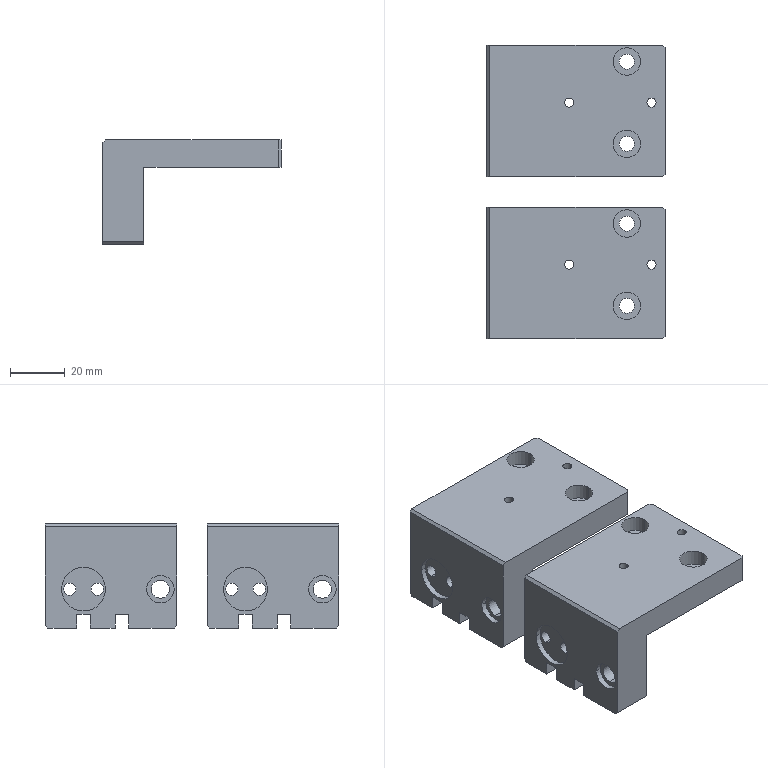NC program | NX | posted with a generic post | part box 65 x 107 x 38 mm
Whole program:
N10 G17 G21 G94 G90
(HOLE_MILLING_COPY_1 , TOOL : D6)
N12 T12 M6
N14 G54
N16 G17 G0 G90 X-18. Y-4.8 B0. C0. S9500 M3
N18 G43 Z30. H12
N20 Z-49.5
N22 G94 G3 X-16.75 Y-6.05 R1.25 F500.
N24 X-15.5 Y-4.8 R1.25
N26 X-15.5 Y-4.8 Z-50. I-2.5 J0.
N28 X-15.5 Y-4.8 Z-50.5 I-2.5 J0.
N30 X-15.5 Y-4.8 Z-51. I-2.5 J0.
N32 X-15.5 Y-4.8 Z-51.5 I-2.5 J0.
N34 X-15.5 Y-4.8 Z-52. I-2.5 J0.
N36 X-15.5 Y-4.8 Z-52.5 I-2.5 J0.
N38 X-15.5 Y-4.8 Z-53. I-2.5 J0.
N40 X-15.5 Y-4.8 Z-53.5 I-2.5 J0.
N42 X-15.5 Y-4.8 Z-54. I-2.5 J0.
N44 X-15.5 Y-4.8 Z-54.5 I-2.5 J0.
N46 X-15.5 Y-4.8 Z-55. I-2.5 J0.
N48 X-15.5 Y-4.8 Z-55.5 I-2.5 J0.
N50 X-15.5 Y-4.8 Z-56. I-2.5 J0.
N52 X-15.5 Y-4.8 Z-56.5 I-2.5 J0.
N54 X-20.023 Y-6.269 Z-56.8 R-2.5
N56 X-16.531 Y-6.823 R2.5
N58 X-20.023 Y-6.269 R-2.5
N60 X-18.277 Y-6.546 R1.25
N62 X-18. Y-4.8 R1.25
N64 G0 Z30.
(HOLE_MILLING_COPY_1_COPY , TOOL : D6)
N66 X5.
N68 Z-49.5
N70 G3 X5.5 Y-5.3 R0.5
N72 X6. Y-4.8 R0.5
N74 X6. Y-4.8 Z-50. I-1. J0.
N76 X6. Y-4.8 Z-50.5 I-1. J0.
N78 X6. Y-4.8 Z-51. I-1. J0.
N80 X6. Y-4.8 Z-51.5 I-1. J0.
N82 X6. Y-4.8 Z-52. I-1. J0.
N84 X6. Y-4.8 Z-52.5 I-1. J0.
N86 X6. Y-4.8 Z-53. I-1. J0.
N88 X6. Y-4.8 Z-53.5 I-1. J0.
N90 X6. Y-4.8 Z-54. I-1. J0.
N92 X6. Y-4.8 Z-54.5 I-1. J0.
N94 X5.309 Y-3.849 Z-54.6 R1.
N96 X4.049 Y-4.491 R1.
N98 X5.309 Y-3.849 R-1.
N100 X4.679 Y-4.17 R0.5
N102 X5. Y-4.8 R0.5
N104 G0 Z30.
N106 X15.
N108 Z-49.5
N110 G3 X15.5 Y-5.3 R0.5
N112 X16. Y-4.8 R0.5
N114 X16. Y-4.8 Z-50. I-1. J0.
N116 X16. Y-4.8 Z-50.5 I-1. J0.
N118 X16. Y-4.8 Z-51. I-1. J0.
N120 X16. Y-4.8 Z-51.5 I-1. J0.
N122 X16. Y-4.8 Z-52. I-1. J0.
N124 X16. Y-4.8 Z-52.5 I-1. J0.
N126 X16. Y-4.8 Z-53. I-1. J0.
N128 X16. Y-4.8 Z-53.5 I-1. J0.
N130 X16. Y-4.8 Z-54. I-1. J0.
N132 X16. Y-4.8 Z-54.5 I-1. J0.
N134 X15.309 Y-3.849 Z-54.6 R1.
N136 X14.049 Y-4.491 R1.
N138 X15.309 Y-3.849 R-1.
N140 X14.679 Y-4.17 R0.5
N142 X15. Y-4.8 R0.5
N144 G0 Z30.
N146 M5
N148 M2